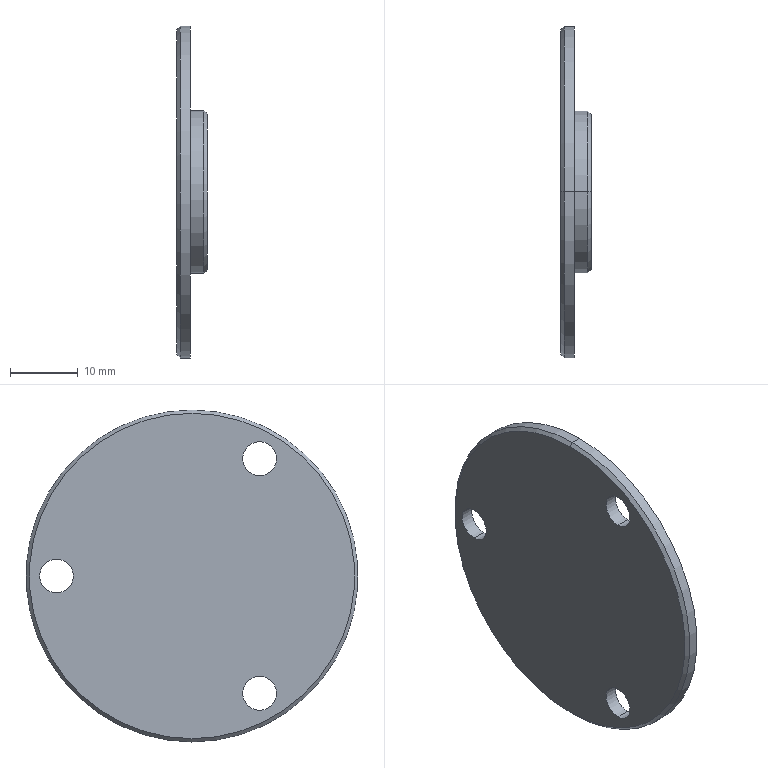Part | SolidWorks | features ICE 3, Chamfer 1, Extrusion 1 | 1 solid | 20 faces | box 4.5 x 49 x 49 mm | volume 3890 mm3 | cylinder 12 | cone 4 | plane 4 | commonest cylinder face diameters 5 x6 21 x2 24 x2 49 x2
STEP:
#1=CARTESIAN_POINT('',(0.,0.,24.));
#2=VERTEX_POINT('',#1);
#3=CARTESIAN_POINT('',(0.,0.,-24.));
#4=VERTEX_POINT('',#3);
#5=CARTESIAN_POINT('',(0.,0.,0.));
#6=DIRECTION('',(-1.,0.,0.));
#7=DIRECTION('',(0.,0.,-1.));
#8=AXIS2_PLACEMENT_3D('',#5,#6,#7);
#9=CIRCLE('',#8,24.);
#10=EDGE_CURVE('',#2,#4,#9,.T.);
#11=ORIENTED_EDGE('',*,*,#10,.F.);
#12=CARTESIAN_POINT('',(0.5,0.,24.5));
#13=VERTEX_POINT('',#12);
#14=CARTESIAN_POINT('',(0.5,0.,24.5));
#15=DIRECTION('',(0.7071,0.,0.7071));
#16=VECTOR('',#15,1000.);
#17=LINE('',#14,#16);
#18=EDGE_CURVE('',#2,#13,#17,.T.);
#19=ORIENTED_EDGE('',*,*,#18,.T.);
#20=CARTESIAN_POINT('',(0.5,0.,-24.5));
#21=VERTEX_POINT('',#20);
#22=CARTESIAN_POINT('',(0.5,0.,0.));
#23=DIRECTION('',(1.,0.,0.));
#24=DIRECTION('',(0.,0.,-1.));
#25=AXIS2_PLACEMENT_3D('',#22,#23,#24);
#26=CIRCLE('',#25,24.5);
#27=EDGE_CURVE('',#21,#13,#26,.T.);
#28=ORIENTED_EDGE('',*,*,#27,.F.);
#29=CARTESIAN_POINT('',(0.5,0.,-24.5));
#30=DIRECTION('',(0.7071,0.,-0.7071));
#31=VECTOR('',#30,1000.);
#32=LINE('',#29,#31);
#33=EDGE_CURVE('',#4,#21,#32,.T.);
#34=ORIENTED_EDGE('',*,*,#33,.F.);
#35=EDGE_LOOP('',(#11,#19,#28,#34));
#36=FACE_OUTER_BOUND('',#35,.T.);
#37=CARTESIAN_POINT('',(0.5,0.,0.));
#38=DIRECTION('',(1.,0.,0.));
#39=DIRECTION('',(0.,0.,-1.));
#40=AXIS2_PLACEMENT_3D('',#37,#38,#39);
#41=CONICAL_SURFACE('',#40,24.5,0.7854);
#42=ADVANCED_FACE('',(#36),#41,.T.);
#43=CARTESIAN_POINT('',(4.5,0.,-11.5));
#44=VERTEX_POINT('',#43);
#45=CARTESIAN_POINT('',(4.5,0.,11.5));
#46=VERTEX_POINT('',#45);
#47=CARTESIAN_POINT('',(4.5,0.,0.));
#48=DIRECTION('',(1.,0.,0.));
#49=DIRECTION('',(0.,0.,-1.));
#50=AXIS2_PLACEMENT_3D('',#47,#48,#49);
#51=CIRCLE('',#50,11.5);
#52=EDGE_CURVE('',#44,#46,#51,.T.);
#53=ORIENTED_EDGE('',*,*,#52,.F.);
#54=CARTESIAN_POINT('',(4.,0.,-12.));
#55=VERTEX_POINT('',#54);
#56=CARTESIAN_POINT('',(4.5,0.,-11.5));
#57=DIRECTION('',(-0.7071,0.,-0.7071));
#58=VECTOR('',#57,1000.);
#59=LINE('',#56,#58);
#60=EDGE_CURVE('',#44,#55,#59,.T.);
#61=ORIENTED_EDGE('',*,*,#60,.T.);
#62=CARTESIAN_POINT('',(4.,0.,12.));
#63=VERTEX_POINT('',#62);
#64=CARTESIAN_POINT('',(4.,0.,0.));
#65=DIRECTION('',(-1.,0.,0.));
#66=DIRECTION('',(0.,0.,-1.));
#67=AXIS2_PLACEMENT_3D('',#64,#65,#66);
#68=CIRCLE('',#67,12.);
#69=EDGE_CURVE('',#63,#55,#68,.T.);
#70=ORIENTED_EDGE('',*,*,#69,.F.);
#71=CARTESIAN_POINT('',(4.5,0.,11.5));
#72=DIRECTION('',(-0.7071,0.,0.7071));
#73=VECTOR('',#72,1000.);
#74=LINE('',#71,#73);
#75=EDGE_CURVE('',#46,#63,#74,.T.);
#76=ORIENTED_EDGE('',*,*,#75,.F.);
#77=EDGE_LOOP('',(#53,#61,#70,#76));
#78=FACE_OUTER_BOUND('',#77,.T.);
#79=CARTESIAN_POINT('',(4.5,0.,0.));
#80=DIRECTION('',(-1.,0.,0.));
#81=DIRECTION('',(0.,0.,1.));
#82=AXIS2_PLACEMENT_3D('',#79,#80,#81);
#83=CONICAL_SURFACE('',#82,11.5,0.7854);
#84=ADVANCED_FACE('',(#78),#83,.T.);
#85=CARTESIAN_POINT('',(2.,20.,2.5));
#86=VERTEX_POINT('',#85);
#87=CARTESIAN_POINT('',(2.,20.,-2.5));
#88=VERTEX_POINT('',#87);
#89=CARTESIAN_POINT('',(2.,20.,0.));
#90=DIRECTION('',(1.,0.,0.));
#91=DIRECTION('',(0.,0.,-1.));
#92=AXIS2_PLACEMENT_3D('',#89,#90,#91);
#93=CIRCLE('',#92,2.5);
#94=EDGE_CURVE('',#86,#88,#93,.T.);
#95=ORIENTED_EDGE('',*,*,#94,.T.);
#96=CARTESIAN_POINT('',(0.,20.,-2.5));
#97=VERTEX_POINT('',#96);
#98=CARTESIAN_POINT('',(2.5,20.,-2.5));
#99=DIRECTION('',(-1.,0.,0.));
#100=VECTOR('',#99,1000.);
#101=LINE('',#98,#100);
#102=EDGE_CURVE('',#88,#97,#101,.T.);
#103=ORIENTED_EDGE('',*,*,#102,.T.);
#104=CARTESIAN_POINT('',(0.,20.,2.5));
#105=VERTEX_POINT('',#104);
#106=CARTESIAN_POINT('',(0.,20.,0.));
#107=DIRECTION('',(-1.,0.,0.));
#108=DIRECTION('',(0.,0.,1.));
#109=AXIS2_PLACEMENT_3D('',#106,#107,#108);
#110=CIRCLE('',#109,2.5);
#111=EDGE_CURVE('',#97,#105,#110,.T.);
#112=ORIENTED_EDGE('',*,*,#111,.T.);
#113=CARTESIAN_POINT('',(2.5,20.,2.5));
#114=DIRECTION('',(-1.,0.,0.));
#115=VECTOR('',#114,1000.);
#116=LINE('',#113,#115);
#117=EDGE_CURVE('',#86,#105,#116,.T.);
#118=ORIENTED_EDGE('',*,*,#117,.F.);
#119=EDGE_LOOP('',(#95,#103,#112,#118));
#120=FACE_OUTER_BOUND('',#119,.T.);
#121=CARTESIAN_POINT('',(2.5,20.,0.));
#122=DIRECTION('',(-1.,0.,0.));
#123=DIRECTION('',(0.,0.,1.));
#124=AXIS2_PLACEMENT_3D('',#121,#122,#123);
#125=CYLINDRICAL_SURFACE('',#124,2.5);
#126=ADVANCED_FACE('',(#120),#125,.F.);
#127=CARTESIAN_POINT('',(2.,-10.,19.821));
#128=VERTEX_POINT('',#127);
#129=CARTESIAN_POINT('',(2.,-10.,14.821));
#130=VERTEX_POINT('',#129);
#131=CARTESIAN_POINT('',(2.,-10.,17.321));
#132=DIRECTION('',(1.,0.,0.));
#133=DIRECTION('',(0.,0.,-1.));
#134=AXIS2_PLACEMENT_3D('',#131,#132,#133);
#135=CIRCLE('',#134,2.5);
#136=EDGE_CURVE('',#128,#130,#135,.T.);
#137=ORIENTED_EDGE('',*,*,#136,.T.);
#138=CARTESIAN_POINT('',(0.,-10.,14.821));
#139=VERTEX_POINT('',#138);
#140=CARTESIAN_POINT('',(2.5,-10.,14.821));
#141=DIRECTION('',(-1.,0.,0.));
#142=VECTOR('',#141,1000.);
#143=LINE('',#140,#142);
#144=EDGE_CURVE('',#130,#139,#143,.T.);
#145=ORIENTED_EDGE('',*,*,#144,.T.);
#146=CARTESIAN_POINT('',(0.,-10.,19.821));
#147=VERTEX_POINT('',#146);
#148=CARTESIAN_POINT('',(0.,-10.,17.321));
#149=DIRECTION('',(-1.,0.,0.));
#150=DIRECTION('',(0.,0.,1.));
#151=AXIS2_PLACEMENT_3D('',#148,#149,#150);
#152=CIRCLE('',#151,2.5);
#153=EDGE_CURVE('',#139,#147,#152,.T.);
#154=ORIENTED_EDGE('',*,*,#153,.T.);
#155=CARTESIAN_POINT('',(2.5,-10.,19.821));
#156=DIRECTION('',(-1.,0.,0.));
#157=VECTOR('',#156,1000.);
#158=LINE('',#155,#157);
#159=EDGE_CURVE('',#128,#147,#158,.T.);
#160=ORIENTED_EDGE('',*,*,#159,.F.);
#161=EDGE_LOOP('',(#137,#145,#154,#160));
#162=FACE_OUTER_BOUND('',#161,.T.);
#163=CARTESIAN_POINT('',(2.5,-10.,17.321));
#164=DIRECTION('',(-1.,0.,0.));
#165=DIRECTION('',(0.,0.,1.));
#166=AXIS2_PLACEMENT_3D('',#163,#164,#165);
#167=CYLINDRICAL_SURFACE('',#166,2.5);
#168=ADVANCED_FACE('',(#162),#167,.F.);
#169=CARTESIAN_POINT('',(2.,-10.,-14.821));
#170=VERTEX_POINT('',#169);
#171=CARTESIAN_POINT('',(2.,-10.,-19.821));
#172=VERTEX_POINT('',#171);
#173=CARTESIAN_POINT('',(2.,-10.,-17.321));
#174=DIRECTION('',(1.,0.,0.));
#175=DIRECTION('',(0.,0.,-1.));
#176=AXIS2_PLACEMENT_3D('',#173,#174,#175);
#177=CIRCLE('',#176,2.5);
#178=EDGE_CURVE('',#170,#172,#177,.T.);
#179=ORIENTED_EDGE('',*,*,#178,.T.);
#180=CARTESIAN_POINT('',(0.,-10.,-19.821));
#181=VERTEX_POINT('',#180);
#182=CARTESIAN_POINT('',(2.5,-10.,-19.821));
#183=DIRECTION('',(-1.,0.,0.));
#184=VECTOR('',#183,1000.);
#185=LINE('',#182,#184);
#186=EDGE_CURVE('',#172,#181,#185,.T.);
#187=ORIENTED_EDGE('',*,*,#186,.T.);
#188=CARTESIAN_POINT('',(0.,-10.,-14.821));
#189=VERTEX_POINT('',#188);
#190=CARTESIAN_POINT('',(0.,-10.,-17.321));
#191=DIRECTION('',(-1.,0.,0.));
#192=DIRECTION('',(0.,0.,1.));
#193=AXIS2_PLACEMENT_3D('',#190,#191,#192);
#194=CIRCLE('',#193,2.5);
#195=EDGE_CURVE('',#181,#189,#194,.T.);
#196=ORIENTED_EDGE('',*,*,#195,.T.);
#197=CARTESIAN_POINT('',(2.5,-10.,-14.821));
#198=DIRECTION('',(-1.,0.,0.));
#199=VECTOR('',#198,1000.);
#200=LINE('',#197,#199);
#201=EDGE_CURVE('',#170,#189,#200,.T.);
#202=ORIENTED_EDGE('',*,*,#201,.F.);
#203=EDGE_LOOP('',(#179,#187,#196,#202));
#204=FACE_OUTER_BOUND('',#203,.T.);
#205=CARTESIAN_POINT('',(2.5,-10.,-17.321));
#206=DIRECTION('',(-1.,0.,0.));
#207=DIRECTION('',(0.,0.,1.));
#208=AXIS2_PLACEMENT_3D('',#205,#206,#207);
#209=CYLINDRICAL_SURFACE('',#208,2.5);
#210=ADVANCED_FACE('',(#204),#209,.F.);
#211=CARTESIAN_POINT('',(4.5,0.,-10.5));
#212=VERTEX_POINT('',#211);
#213=CARTESIAN_POINT('',(4.5,0.,10.5));
#214=VERTEX_POINT('',#213);
#215=CARTESIAN_POINT('',(4.5,0.,0.));
#216=DIRECTION('',(-1.,0.,0.));
#217=DIRECTION('',(0.,0.,-1.));
#218=AXIS2_PLACEMENT_3D('',#215,#216,#217);
#219=CIRCLE('',#218,10.5);
#220=EDGE_CURVE('',#212,#214,#219,.T.);
#221=ORIENTED_EDGE('',*,*,#220,.F.);
#222=CARTESIAN_POINT('',(2.,0.,-10.5));
#223=VERTEX_POINT('',#222);
#224=CARTESIAN_POINT('',(4.5,0.,-10.5));
#225=DIRECTION('',(-1.,0.,0.));
#226=VECTOR('',#225,1000.);
#227=LINE('',#224,#226);
#228=EDGE_CURVE('',#212,#223,#227,.T.);
#229=ORIENTED_EDGE('',*,*,#228,.T.);
#230=CARTESIAN_POINT('',(2.,0.,10.5));
#231=VERTEX_POINT('',#230);
#232=CARTESIAN_POINT('',(2.,0.,0.));
#233=DIRECTION('',(1.,0.,0.));
#234=DIRECTION('',(0.,0.,-1.));
#235=AXIS2_PLACEMENT_3D('',#232,#233,#234);
#236=CIRCLE('',#235,10.5);
#237=EDGE_CURVE('',#231,#223,#236,.T.);
#238=ORIENTED_EDGE('',*,*,#237,.F.);
#239=CARTESIAN_POINT('',(4.5,0.,10.5));
#240=DIRECTION('',(-1.,0.,0.));
#241=VECTOR('',#240,1000.);
#242=LINE('',#239,#241);
#243=EDGE_CURVE('',#214,#231,#242,.T.);
#244=ORIENTED_EDGE('',*,*,#243,.F.);
#245=EDGE_LOOP('',(#221,#229,#238,#244));
#246=FACE_OUTER_BOUND('',#245,.T.);
#247=CARTESIAN_POINT('',(4.5,0.,0.));
#248=DIRECTION('',(-1.,0.,0.));
#249=DIRECTION('',(0.,0.,1.));
#250=AXIS2_PLACEMENT_3D('',#247,#248,#249);
#251=CYLINDRICAL_SURFACE('',#250,10.5);
#252=ADVANCED_FACE('',(#246),#251,.F.);
#253=ORIENTED_EDGE('',*,*,#69,.T.);
#254=CARTESIAN_POINT('',(2.,0.,-12.));
#255=VERTEX_POINT('',#254);
#256=CARTESIAN_POINT('',(4.5,0.,-12.));
#257=DIRECTION('',(-1.,0.,0.));
#258=VECTOR('',#257,1000.);
#259=LINE('',#256,#258);
#260=EDGE_CURVE('',#55,#255,#259,.T.);
#261=ORIENTED_EDGE('',*,*,#260,.T.);
#262=CARTESIAN_POINT('',(2.,0.,12.));
#263=VERTEX_POINT('',#262);
#264=CARTESIAN_POINT('',(2.,0.,0.));
#265=DIRECTION('',(1.,0.,0.));
#266=DIRECTION('',(0.,0.,-1.));
#267=AXIS2_PLACEMENT_3D('',#264,#265,#266);
#268=CIRCLE('',#267,12.);
#269=EDGE_CURVE('',#255,#263,#268,.T.);
#270=ORIENTED_EDGE('',*,*,#269,.T.);
#271=CARTESIAN_POINT('',(4.5,0.,12.));
#272=DIRECTION('',(-1.,0.,0.));
#273=VECTOR('',#272,1000.);
#274=LINE('',#271,#273);
#275=EDGE_CURVE('',#63,#263,#274,.T.);
#276=ORIENTED_EDGE('',*,*,#275,.F.);
#277=EDGE_LOOP('',(#253,#261,#270,#276));
#278=FACE_OUTER_BOUND('',#277,.T.);
#279=CARTESIAN_POINT('',(4.5,0.,0.));
#280=DIRECTION('',(-1.,0.,0.));
#281=DIRECTION('',(0.,0.,1.));
#282=AXIS2_PLACEMENT_3D('',#279,#280,#281);
#283=CYLINDRICAL_SURFACE('',#282,12.);
#284=ADVANCED_FACE('',(#278),#283,.T.);
#285=CARTESIAN_POINT('',(2.,0.,-24.5));
#286=VERTEX_POINT('',#285);
#287=CARTESIAN_POINT('',(2.,0.,24.5));
#288=VERTEX_POINT('',#287);
#289=CARTESIAN_POINT('',(2.,0.,0.));
#290=DIRECTION('',(1.,0.,0.));
#291=DIRECTION('',(0.,0.,-1.));
#292=AXIS2_PLACEMENT_3D('',#289,#290,#291);
#293=CIRCLE('',#292,24.5);
#294=EDGE_CURVE('',#286,#288,#293,.T.);
#295=ORIENTED_EDGE('',*,*,#294,.F.);
#296=CARTESIAN_POINT('',(2.,0.,-24.5));
#297=DIRECTION('',(-1.,0.,0.));
#298=VECTOR('',#297,1000.);
#299=LINE('',#296,#298);
#300=EDGE_CURVE('',#286,#21,#299,.T.);
#301=ORIENTED_EDGE('',*,*,#300,.T.);
#302=ORIENTED_EDGE('',*,*,#27,.T.);
#303=CARTESIAN_POINT('',(2.,0.,24.5));
#304=DIRECTION('',(-1.,0.,0.));
#305=VECTOR('',#304,1000.);
#306=LINE('',#303,#305);
#307=EDGE_CURVE('',#288,#13,#306,.T.);
#308=ORIENTED_EDGE('',*,*,#307,.F.);
#309=EDGE_LOOP('',(#295,#301,#302,#308));
#310=FACE_OUTER_BOUND('',#309,.T.);
#311=CARTESIAN_POINT('',(2.,0.,0.));
#312=DIRECTION('',(-1.,0.,0.));
#313=DIRECTION('',(0.,0.,1.));
#314=AXIS2_PLACEMENT_3D('',#311,#312,#313);
#315=CYLINDRICAL_SURFACE('',#314,24.5);
#316=ADVANCED_FACE('',(#310),#315,.T.);
#317=ORIENTED_EDGE('',*,*,#300,.F.);
#318=CARTESIAN_POINT('',(2.,0.,0.));
#319=DIRECTION('',(1.,0.,0.));
#320=DIRECTION('',(0.,0.,-1.));
#321=AXIS2_PLACEMENT_3D('',#318,#319,#320);
#322=CIRCLE('',#321,24.5);
#323=EDGE_CURVE('',#288,#286,#322,.T.);
#324=ORIENTED_EDGE('',*,*,#323,.F.);
#325=ORIENTED_EDGE('',*,*,#307,.T.);
#326=CARTESIAN_POINT('',(0.5,0.,0.));
#327=DIRECTION('',(1.,0.,0.));
#328=DIRECTION('',(0.,0.,-1.));
#329=AXIS2_PLACEMENT_3D('',#326,#327,#328);
#330=CIRCLE('',#329,24.5);
#331=EDGE_CURVE('',#13,#21,#330,.T.);
#332=ORIENTED_EDGE('',*,*,#331,.T.);
#333=EDGE_LOOP('',(#317,#324,#325,#332));
#334=FACE_OUTER_BOUND('',#333,.T.);
#335=CARTESIAN_POINT('',(2.,0.,0.));
#336=DIRECTION('',(-1.,0.,0.));
#337=DIRECTION('',(0.,0.,1.));
#338=AXIS2_PLACEMENT_3D('',#335,#336,#337);
#339=CYLINDRICAL_SURFACE('',#338,24.5);
#340=ADVANCED_FACE('',(#334),#339,.T.);
#341=ORIENTED_EDGE('',*,*,#94,.F.);
#342=CARTESIAN_POINT('',(2.,20.,0.));
#343=DIRECTION('',(1.,0.,0.));
#344=DIRECTION('',(0.,0.,-1.));
#345=AXIS2_PLACEMENT_3D('',#342,#343,#344);
#346=CIRCLE('',#345,2.5);
#347=EDGE_CURVE('',#88,#86,#346,.T.);
#348=ORIENTED_EDGE('',*,*,#347,.F.);
#349=EDGE_LOOP('',(#341,#348));
#350=FACE_BOUND('',#349,.T.);
#351=ORIENTED_EDGE('',*,*,#136,.F.);
#352=CARTESIAN_POINT('',(2.,-10.,17.321));
#353=DIRECTION('',(1.,0.,0.));
#354=DIRECTION('',(0.,0.,-1.));
#355=AXIS2_PLACEMENT_3D('',#352,#353,#354);
#356=CIRCLE('',#355,2.5);
#357=EDGE_CURVE('',#130,#128,#356,.T.);
#358=ORIENTED_EDGE('',*,*,#357,.F.);
#359=EDGE_LOOP('',(#351,#358));
#360=FACE_BOUND('',#359,.T.);
#361=ORIENTED_EDGE('',*,*,#178,.F.);
#362=CARTESIAN_POINT('',(2.,-10.,-17.321));
#363=DIRECTION('',(1.,0.,0.));
#364=DIRECTION('',(0.,0.,-1.));
#365=AXIS2_PLACEMENT_3D('',#362,#363,#364);
#366=CIRCLE('',#365,2.5);
#367=EDGE_CURVE('',#172,#170,#366,.T.);
#368=ORIENTED_EDGE('',*,*,#367,.F.);
#369=EDGE_LOOP('',(#361,#368));
#370=FACE_BOUND('',#369,.T.);
#371=CARTESIAN_POINT('',(2.,0.,0.));
#372=DIRECTION('',(1.,0.,0.));
#373=DIRECTION('',(0.,0.,-1.));
#374=AXIS2_PLACEMENT_3D('',#371,#372,#373);
#375=CIRCLE('',#374,12.);
#376=EDGE_CURVE('',#263,#255,#375,.T.);
#377=ORIENTED_EDGE('',*,*,#376,.F.);
#378=ORIENTED_EDGE('',*,*,#269,.F.);
#379=EDGE_LOOP('',(#377,#378));
#380=FACE_BOUND('',#379,.T.);
#381=ORIENTED_EDGE('',*,*,#323,.T.);
#382=ORIENTED_EDGE('',*,*,#294,.T.);
#383=EDGE_LOOP('',(#381,#382));
#384=FACE_OUTER_BOUND('',#383,.T.);
#385=CARTESIAN_POINT('',(2.,0.,0.));
#386=DIRECTION('',(1.,0.,0.));
#387=DIRECTION('',(0.,0.,-1.));
#388=AXIS2_PLACEMENT_3D('',#385,#386,#387);
#389=PLANE('',#388);
#390=ADVANCED_FACE('',(#350,#360,#370,#380,#384),#389,.T.);
#391=CARTESIAN_POINT('',(0.,0.,0.));
#392=DIRECTION('',(-1.,0.,0.));
#393=DIRECTION('',(0.,0.,-1.));
#394=AXIS2_PLACEMENT_3D('',#391,#392,#393);
#395=CIRCLE('',#394,24.);
#396=EDGE_CURVE('',#4,#2,#395,.T.);
#397=ORIENTED_EDGE('',*,*,#396,.T.);
#398=ORIENTED_EDGE('',*,*,#10,.T.);
#399=EDGE_LOOP('',(#397,#398));
#400=FACE_OUTER_BOUND('',#399,.T.);
#401=CARTESIAN_POINT('',(0.,20.,0.));
#402=DIRECTION('',(-1.,0.,0.));
#403=DIRECTION('',(0.,0.,1.));
#404=AXIS2_PLACEMENT_3D('',#401,#402,#403);
#405=CIRCLE('',#404,2.5);
#406=EDGE_CURVE('',#105,#97,#405,.T.);
#407=ORIENTED_EDGE('',*,*,#406,.F.);
#408=ORIENTED_EDGE('',*,*,#111,.F.);
#409=EDGE_LOOP('',(#407,#408));
#410=FACE_BOUND('',#409,.T.);
#411=CARTESIAN_POINT('',(0.,-10.,17.321));
#412=DIRECTION('',(-1.,0.,0.));
#413=DIRECTION('',(0.,0.,1.));
#414=AXIS2_PLACEMENT_3D('',#411,#412,#413);
#415=CIRCLE('',#414,2.5);
#416=EDGE_CURVE('',#147,#139,#415,.T.);
#417=ORIENTED_EDGE('',*,*,#416,.F.);
#418=ORIENTED_EDGE('',*,*,#153,.F.);
#419=EDGE_LOOP('',(#417,#418));
#420=FACE_BOUND('',#419,.T.);
#421=CARTESIAN_POINT('',(0.,-10.,-17.321));
#422=DIRECTION('',(-1.,0.,0.));
#423=DIRECTION('',(0.,0.,1.));
#424=AXIS2_PLACEMENT_3D('',#421,#422,#423);
#425=CIRCLE('',#424,2.5);
#426=EDGE_CURVE('',#189,#181,#425,.T.);
#427=ORIENTED_EDGE('',*,*,#426,.F.);
#428=ORIENTED_EDGE('',*,*,#195,.F.);
#429=EDGE_LOOP('',(#427,#428));
#430=FACE_BOUND('',#429,.T.);
#431=CARTESIAN_POINT('',(0.,0.,0.));
#432=DIRECTION('',(1.,0.,0.));
#433=DIRECTION('',(0.,0.,-1.));
#434=AXIS2_PLACEMENT_3D('',#431,#432,#433);
#435=PLANE('',#434);
#436=ADVANCED_FACE('',(#400,#410,#420,#430),#435,.F.);
#437=ORIENTED_EDGE('',*,*,#260,.F.);
#438=CARTESIAN_POINT('',(4.,0.,0.));
#439=DIRECTION('',(-1.,0.,0.));
#440=DIRECTION('',(0.,0.,-1.));
#441=AXIS2_PLACEMENT_3D('',#438,#439,#440);
#442=CIRCLE('',#441,12.);
#443=EDGE_CURVE('',#55,#63,#442,.T.);
#444=ORIENTED_EDGE('',*,*,#443,.T.);
#445=ORIENTED_EDGE('',*,*,#275,.T.);
#446=ORIENTED_EDGE('',*,*,#376,.T.);
#447=EDGE_LOOP('',(#437,#444,#445,#446));
#448=FACE_OUTER_BOUND('',#447,.T.);
#449=CARTESIAN_POINT('',(4.5,0.,0.));
#450=DIRECTION('',(-1.,0.,0.));
#451=DIRECTION('',(0.,0.,1.));
#452=AXIS2_PLACEMENT_3D('',#449,#450,#451);
#453=CYLINDRICAL_SURFACE('',#452,12.);
#454=ADVANCED_FACE('',(#448),#453,.T.);
#455=CARTESIAN_POINT('',(4.5,0.,0.));
#456=DIRECTION('',(1.,0.,0.));
#457=DIRECTION('',(0.,0.,-1.));
#458=AXIS2_PLACEMENT_3D('',#455,#456,#457);
#459=CIRCLE('',#458,11.5);
#460=EDGE_CURVE('',#46,#44,#459,.T.);
#461=ORIENTED_EDGE('',*,*,#460,.T.);
#462=ORIENTED_EDGE('',*,*,#52,.T.);
#463=EDGE_LOOP('',(#461,#462));
#464=FACE_OUTER_BOUND('',#463,.T.);
#465=CARTESIAN_POINT('',(4.5,0.,0.));
#466=DIRECTION('',(-1.,0.,0.));
#467=DIRECTION('',(0.,0.,-1.));
#468=AXIS2_PLACEMENT_3D('',#465,#466,#467);
#469=CIRCLE('',#468,10.5);
#470=EDGE_CURVE('',#214,#212,#469,.T.);
#471=ORIENTED_EDGE('',*,*,#470,.T.);
#472=ORIENTED_EDGE('',*,*,#220,.T.);
#473=EDGE_LOOP('',(#471,#472));
#474=FACE_BOUND('',#473,.T.);
#475=CARTESIAN_POINT('',(4.5,0.,0.));
#476=DIRECTION('',(1.,0.,0.));
#477=DIRECTION('',(0.,0.,-1.));
#478=AXIS2_PLACEMENT_3D('',#475,#476,#477);
#479=PLANE('',#478);
#480=ADVANCED_FACE('',(#464,#474),#479,.T.);
#481=ORIENTED_EDGE('',*,*,#228,.F.);
#482=ORIENTED_EDGE('',*,*,#470,.F.);
#483=ORIENTED_EDGE('',*,*,#243,.T.);
#484=CARTESIAN_POINT('',(2.,0.,0.));
#485=DIRECTION('',(1.,0.,0.));
#486=DIRECTION('',(0.,0.,-1.));
#487=AXIS2_PLACEMENT_3D('',#484,#485,#486);
#488=CIRCLE('',#487,10.5);
#489=EDGE_CURVE('',#223,#231,#488,.T.);
#490=ORIENTED_EDGE('',*,*,#489,.F.);
#491=EDGE_LOOP('',(#481,#482,#483,#490));
#492=FACE_OUTER_BOUND('',#491,.T.);
#493=CARTESIAN_POINT('',(4.5,0.,0.));
#494=DIRECTION('',(-1.,0.,0.));
#495=DIRECTION('',(0.,0.,1.));
#496=AXIS2_PLACEMENT_3D('',#493,#494,#495);
#497=CYLINDRICAL_SURFACE('',#496,10.5);
#498=ADVANCED_FACE('',(#492),#497,.F.);
#499=ORIENTED_EDGE('',*,*,#237,.T.);
#500=ORIENTED_EDGE('',*,*,#489,.T.);
#501=EDGE_LOOP('',(#499,#500));
#502=FACE_OUTER_BOUND('',#501,.T.);
#503=CARTESIAN_POINT('',(2.,0.,0.));
#504=DIRECTION('',(1.,0.,0.));
#505=DIRECTION('',(0.,0.,-1.));
#506=AXIS2_PLACEMENT_3D('',#503,#504,#505);
#507=PLANE('',#506);
#508=ADVANCED_FACE('',(#502),#507,.T.);
#509=ORIENTED_EDGE('',*,*,#186,.F.);
#510=ORIENTED_EDGE('',*,*,#367,.T.);
#511=ORIENTED_EDGE('',*,*,#201,.T.);
#512=ORIENTED_EDGE('',*,*,#426,.T.);
#513=EDGE_LOOP('',(#509,#510,#511,#512));
#514=FACE_OUTER_BOUND('',#513,.T.);
#515=CARTESIAN_POINT('',(2.5,-10.,-17.321));
#516=DIRECTION('',(-1.,0.,0.));
#517=DIRECTION('',(0.,0.,1.));
#518=AXIS2_PLACEMENT_3D('',#515,#516,#517);
#519=CYLINDRICAL_SURFACE('',#518,2.5);
#520=ADVANCED_FACE('',(#514),#519,.F.);
#521=ORIENTED_EDGE('',*,*,#144,.F.);
#522=ORIENTED_EDGE('',*,*,#357,.T.);
#523=ORIENTED_EDGE('',*,*,#159,.T.);
#524=ORIENTED_EDGE('',*,*,#416,.T.);
#525=EDGE_LOOP('',(#521,#522,#523,#524));
#526=FACE_OUTER_BOUND('',#525,.T.);
#527=CARTESIAN_POINT('',(2.5,-10.,17.321));
#528=DIRECTION('',(-1.,0.,0.));
#529=DIRECTION('',(0.,0.,1.));
#530=AXIS2_PLACEMENT_3D('',#527,#528,#529);
#531=CYLINDRICAL_SURFACE('',#530,2.5);
#532=ADVANCED_FACE('',(#526),#531,.F.);
#533=ORIENTED_EDGE('',*,*,#102,.F.);
#534=ORIENTED_EDGE('',*,*,#347,.T.);
#535=ORIENTED_EDGE('',*,*,#117,.T.);
#536=ORIENTED_EDGE('',*,*,#406,.T.);
#537=EDGE_LOOP('',(#533,#534,#535,#536));
#538=FACE_OUTER_BOUND('',#537,.T.);
#539=CARTESIAN_POINT('',(2.5,20.,0.));
#540=DIRECTION('',(-1.,0.,0.));
#541=DIRECTION('',(0.,0.,1.));
#542=AXIS2_PLACEMENT_3D('',#539,#540,#541);
#543=CYLINDRICAL_SURFACE('',#542,2.5);
#544=ADVANCED_FACE('',(#538),#543,.F.);
#545=ORIENTED_EDGE('',*,*,#60,.F.);
#546=ORIENTED_EDGE('',*,*,#460,.F.);
#547=ORIENTED_EDGE('',*,*,#75,.T.);
#548=ORIENTED_EDGE('',*,*,#443,.F.);
#549=EDGE_LOOP('',(#545,#546,#547,#548));
#550=FACE_OUTER_BOUND('',#549,.T.);
#551=CARTESIAN_POINT('',(4.5,0.,0.));
#552=DIRECTION('',(-1.,0.,0.));
#553=DIRECTION('',(0.,0.,1.));
#554=AXIS2_PLACEMENT_3D('',#551,#552,#553);
#555=CONICAL_SURFACE('',#554,11.5,0.7854);
#556=ADVANCED_FACE('',(#550),#555,.T.);
#557=ORIENTED_EDGE('',*,*,#18,.F.);
#558=ORIENTED_EDGE('',*,*,#396,.F.);
#559=ORIENTED_EDGE('',*,*,#33,.T.);
#560=ORIENTED_EDGE('',*,*,#331,.F.);
#561=EDGE_LOOP('',(#557,#558,#559,#560));
#562=FACE_OUTER_BOUND('',#561,.T.);
#563=CARTESIAN_POINT('',(0.5,0.,0.));
#564=DIRECTION('',(1.,0.,0.));
#565=DIRECTION('',(0.,0.,-1.));
#566=AXIS2_PLACEMENT_3D('',#563,#564,#565);
#567=CONICAL_SURFACE('',#566,24.5,0.7854);
#568=ADVANCED_FACE('',(#562),#567,.T.);
#569=CLOSED_SHELL('',(#42,#84,#126,#168,#210,#252,#284,#316,#340,#390,#436,#454,#480,#498,#508,#520,#532,#544,#556,#568));
#570=MANIFOLD_SOLID_BREP('',#569);
#571=CARTESIAN_POINT('',(0.,0.,0.));
#572=DIRECTION('',(0.,0.,1.));
#573=DIRECTION('',(1.,0.,0.));
#574=AXIS2_PLACEMENT_3D('',#571,#572,#573);
#575=(LENGTH_UNIT()NAMED_UNIT(*)SI_UNIT(.MILLI.,.METRE.));
#576=UNCERTAINTY_MEASURE_WITH_UNIT(LENGTH_MEASURE(0.00001),#575,'','');
#577=(NAMED_UNIT(*)PLANE_ANGLE_UNIT()SI_UNIT($,.RADIAN.));
#578=(NAMED_UNIT(*)SI_UNIT($,.STERADIAN.)SOLID_ANGLE_UNIT());
#579=(GEOMETRIC_REPRESENTATION_CONTEXT(3)GLOBAL_UNCERTAINTY_ASSIGNED_CONTEXT((#576))GLOBAL_UNIT_ASSIGNED_CONTEXT((#575,#577,#578))REPRESENTATION_CONTEXT('',''));
#580=ADVANCED_BREP_SHAPE_REPRESENTATION('',(#570,#574),#579);